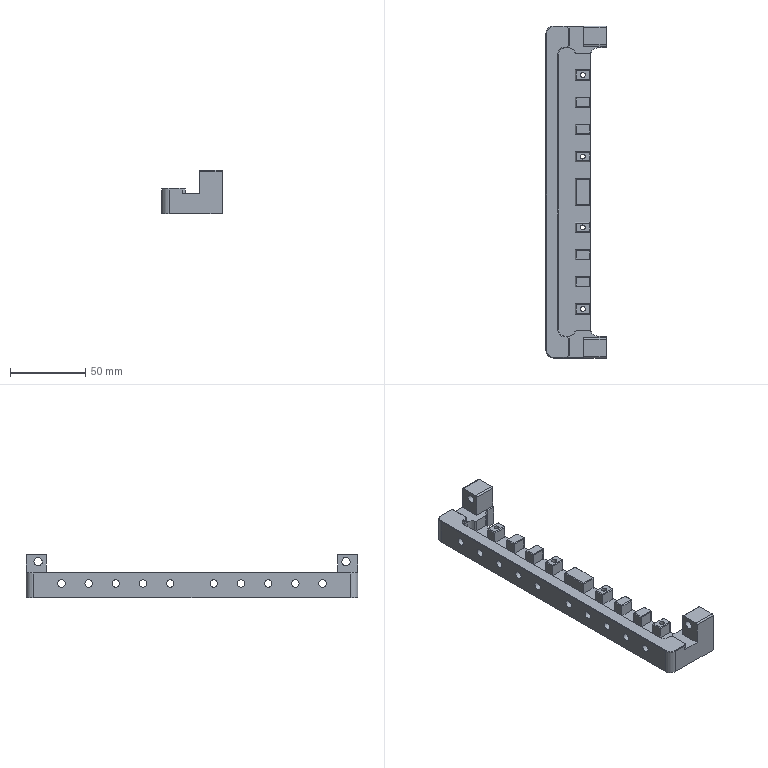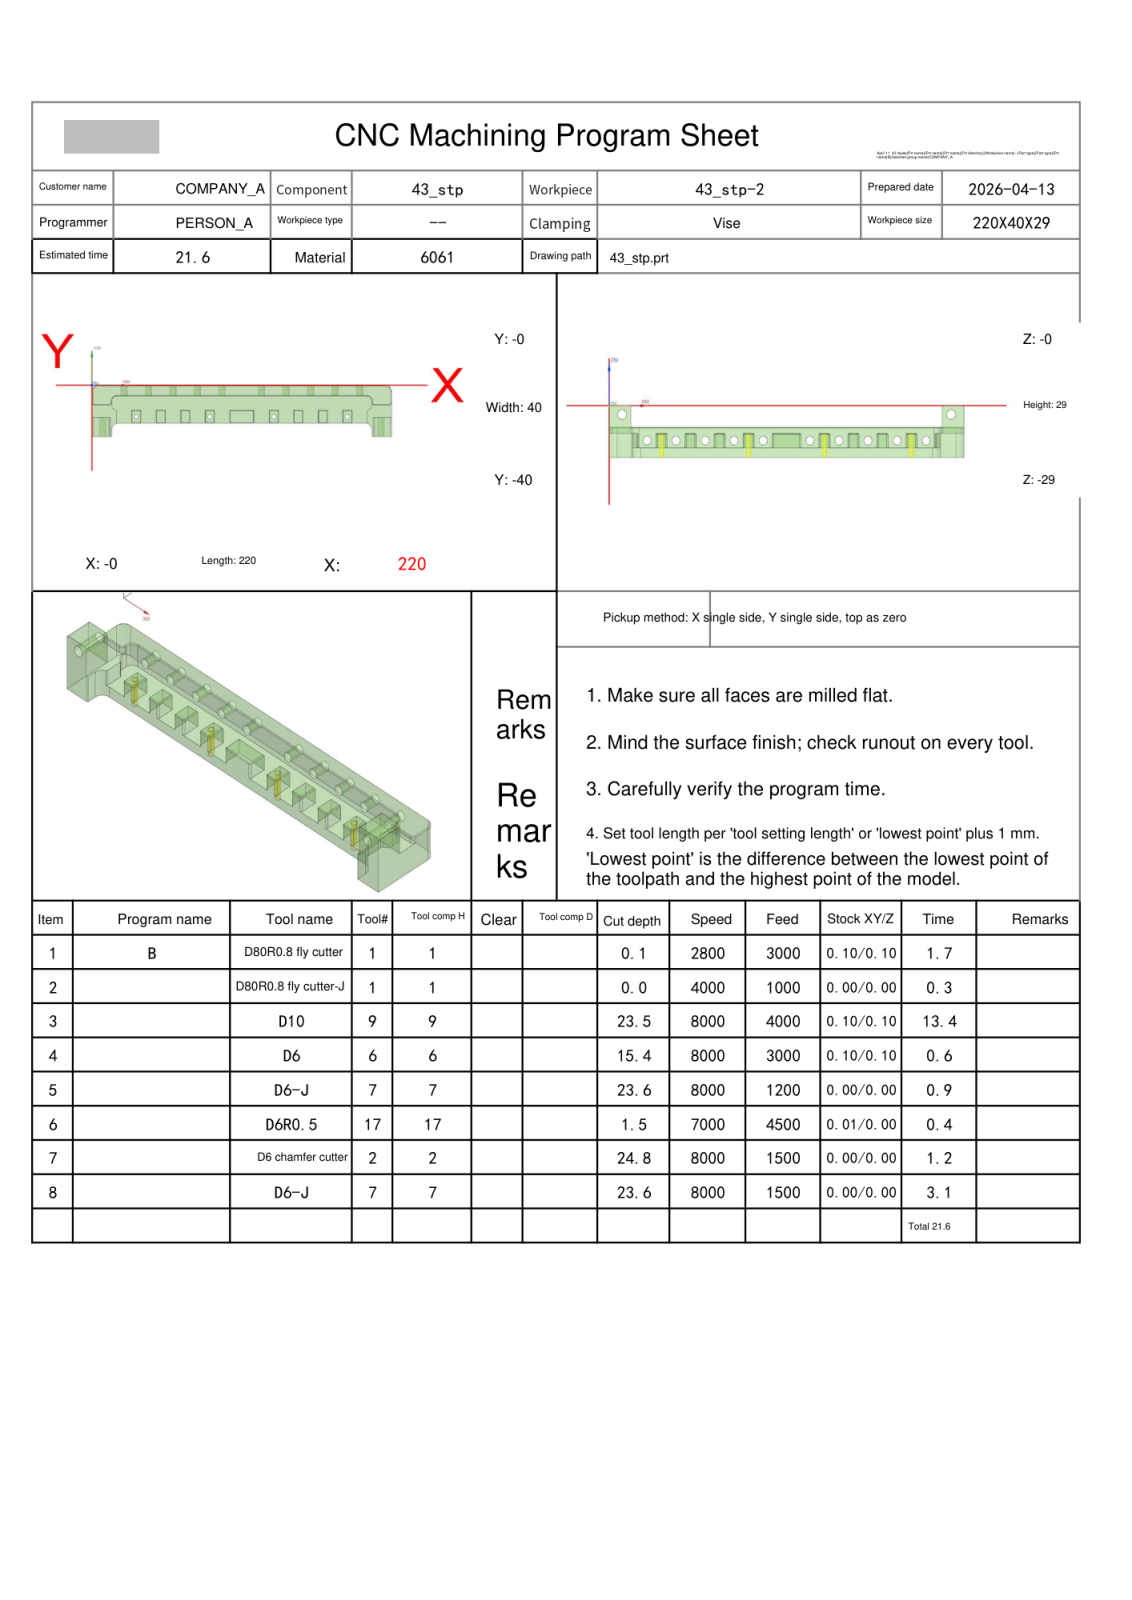NC program | NX | posted by the shop | part box 40 x 220 x 29 mm
Lines 135 to 1312 of 14837:
N3 T09 M06
(D10  D=10. R=0. H=09 ce=0.10 di=0.10)
G00 G90 G54 X110. Y7.5 M03 S8000
G43 H09 Z15.8
M08
Z.905
G01 Z-.595 F4000.
Y4.4
X215.
G02 X224.4 Y-5. I0.0 J-9.4
G01 Y-8.601
X224.9
Y-19.9
X220.403
X201.4
Y-44.9
X200.6
Y-40.296
X198.686 Y-39.233
X196.695 Y-38.128
G02 X196.243 Y-37.538 I.453 J.816
G01 X195.952 Y-36.374
G03 X195.735 Y-35.959 I-.97 J-.243
G02 X195.462 Y-35.581 I1.882 J1.646
G01 X192.575 Y-30.673
G02 X192.23 Y-29.406 I2.155 J1.267
X194.73 Y-26.906 I2.5 J0.0
X196.885 Y-28.138 I0.0 J-2.5
G01 X199.772 Y-33.046
G02 X200.117 Y-34.313 I-2.155 J-1.267
X197.617 Y-36.813 I-2.5 J0.0
X197.203 Y-36.779 I0.0 J2.5
G01 X197.049 Y-36.766
G03 X196.762 Y-36.811 I0.0 J-.934
G01 X195.633 Y-37.175
G02 X195.326 Y-37.223 I-.307 J.952
X194.841 Y-37.098 I0.0 J1.
G01 X190.233 Y-34.539
X189.082 Y-33.9
X185.05
G02 X184.259 Y-33.842 I0.0 J5.4
X183.967 Y-33.79 I.791 J5.342
G01 X173.023 Y-33.792
G02 X171.95 Y-33.9 I-1.073 J5.292
G01 X167.05
G02 X166.259 Y-33.842 I0.0 J5.4
X165.967 Y-33.79 I.79 J5.342
G01 X155.023 Y-33.792
G02 X153.95 Y-33.9 I-1.073 J5.292
G01 X149.05
G02 X148.259 Y-33.842 I0.0 J5.4
X147.967 Y-33.79 I.79 J5.342
G01 X137.023 Y-33.792
G02 X135.95 Y-33.9 I-1.073 J5.292
G01 X131.05
G02 X130.259 Y-33.842 I0.0 J5.4
X129.967 Y-33.79 I.791 J5.342
G01 X119.023 Y-33.792
G02 X117.95 Y-33.9 I-1.073 J5.292
G01 X102.05
G02 X101.259 Y-33.842 I0.0 J5.4
X100.967 Y-33.79 I.79 J5.342
G01 X90.023 Y-33.792
G02 X88.95 Y-33.9 I-1.073 J5.292
G01 X84.05
G02 X83.259 Y-33.842 I0.0 J5.4
X82.967 Y-33.79 I.791 J5.342
G01 X72.023 Y-33.792
G02 X70.95 Y-33.9 I-1.073 J5.292
G01 X66.05
G02 X65.259 Y-33.842 I0.0 J5.4
X64.967 Y-33.79 I.791 J5.342
G01 X54.023 Y-33.792
G02 X52.95 Y-33.9 I-1.073 J5.292
G01 X48.05
G02 X47.26 Y-33.842 I0.0 J5.4
X46.968 Y-33.79 I.79 J5.342
G01 X36.023 Y-33.792
G02 X34.95 Y-33.9 I-1.073 J5.292
G01 X30.918
X25.134 Y-37.112
G02 X24.681 Y-37.229 I-.453 J.816
X24.394 Y-37.184 I0.0 J.934
G01 X23.253 Y-36.816
G03 X22.946 Y-36.767 I-.307 J-.952
G01 X22.786 Y-36.78
G02 X22.383 Y-36.813 I-.402 J2.467
X19.883 Y-34.313 I0.0 J2.5
X20.228 Y-33.046 I2.5 J0.0
G01 X23.115 Y-28.138
G02 X25.27 Y-26.906 I2.155 J-1.267
X27.77 Y-29.406 I0.0 J-2.5
X27.425 Y-30.673 I-2.5 J0.0
G01 X24.538 Y-35.58
G02 X24.257 Y-35.968 I-2.155 J1.267
G03 X24.052 Y-36.359 I.7 J-.618
G01 X23.764 Y-37.51
G02 X23.28 Y-38.141 I-.97 J.243
G01 X21.024 Y-39.394
X19.4 Y-40.296
Y-41.53
X18.6 Y-42.33
Y-19.9
X-4.9
Y-8.602
X-4.4
Y-5.
G02 X5. Y4.4 I9.4 J0.0
G01 X106.966
G02 X107.796 Y3.955 I-.001 J-1.
G01 X112.204 Y-2.655
G03 X113.035 Y-3.1 I.832 J.555
G01 X197.609
G02 X198.311 Y-3.388 I0.0 J-1.
G01 X199.813 Y-4.869
G03 X200.256 Y-5.122 I.702 J.712
G02 X202.109 Y-7.537 I-.647 J-2.415
X200.195 Y-9.967 I-2.5 J0.0
G01 X191.425 Y-12.084
G02 X190.838 Y-12.154 I-.587 J2.43
X188.338 Y-9.654 I0.0 J2.5
X190.252 Y-7.224 I2.5 J0.0
G01 X197.74 Y-5.416
G03 X198.255 Y-5.106 I-.235 J.972
G01 X199.727 Y-3.438
G02 X200.477 Y-3.1 I.75 J-.662
G01 X215.
G02 X216.9 Y-5. I0.0 J-1.9
G01 Y-8.601
G03 X217.32 Y-11.075 I7.5 J0.0
G02 X217.374 Y-11.4 I-.946 J-.325
X216.379 Y-12.4 I-1. J0.0
G01 X201.4
G03 X193.9 Y-19.9 I0.0 J-7.5
G01 Y-26.31
G02 X192.9 Y-27.306 I-1. J.004
X192.455 Y-27.201 I0.0 J1.
G03 X189.082 Y-26.4 I-3.372 J-6.699
G01 X185.357
X185.167 Y-26.381
X184.72 Y-26.29
X172.28
X171.833 Y-26.381
X171.643 Y-26.4
X167.357
X167.167 Y-26.381
X166.72 Y-26.29
X154.28
X153.833 Y-26.381
X153.643 Y-26.4
X149.357
X149.167 Y-26.381
X148.72 Y-26.29
X136.28
X135.833 Y-26.381
X135.643 Y-26.4
X131.357
X131.167 Y-26.381
X130.72 Y-26.29
X118.28
X117.833 Y-26.381
X117.643 Y-26.4
X102.357
X102.167 Y-26.381
X101.72 Y-26.29
X89.28
X88.833 Y-26.381
X88.643 Y-26.4
X84.357
X84.167 Y-26.381
X83.72 Y-26.29
X71.28
X70.833 Y-26.381
X70.643 Y-26.4
X66.357
X66.167 Y-26.381
X65.72 Y-26.29
X53.28
X52.833 Y-26.381
X52.643 Y-26.4
X48.356
X48.167 Y-26.381
X47.72 Y-26.29
X35.28
X34.833 Y-26.381
G02 X34.635 Y-26.401 I-.199 J.981
G01 X34.593 Y-26.4
X30.918
G03 X27.545 Y-27.201 I0.0 J-7.5
G02 X27.1 Y-27.306 I-.445 J.895
X26.1 Y-26.31 I0.0 J1.
G01 Y-19.9
G03 X18.6 Y-12.4 I-7.5 J0.0
G01 X3.622
G02 X2.626 Y-11.4 I.004 J1.
X2.681 Y-11.075 I1. J0.0
G03 X3.1 Y-8.602 I-7.081 J2.473
G01 Y-5.
G02 X5. Y-3.1 I1.9 J0.0
G01 X19.523
G02 X20.273 Y-3.438 I0.0 J-1.
G01 X21.745 Y-5.106
G03 X22.26 Y-5.416 I.75 J.662
G01 X29.748 Y-7.224
G02 X31.662 Y-9.654 I-.587 J-2.43
X29.162 Y-12.154 I-2.5 J0.0
X28.575 Y-12.084 I0.0 J2.5
G01 X19.805 Y-9.967
G02 X17.891 Y-7.537 I.587 J2.43
X19.744 Y-5.122 I2.5 J0.0
G03 X20.187 Y-4.868 I-.259 J.966
G01 X21.689 Y-3.388
G02 X22.391 Y-3.1 I.702 J-.712
G01 X106.965
G02 X107.796 Y-3.545 I-.001 J-1.
G01 X112.204 Y-10.155
G03 X113.035 Y-10.6 I.832 J.555
G01 X187.726
G02 X188.721 Y-11.6 I-.005 J-1.
X188.579 Y-12.115 I-1. J0.0
G03 X186.53 Y-17.929 I12.821 J-7.785
G02 X185.539 Y-18.793 I-.991 J.136
G01 X185.472 Y-18.79
X171.528
X171.08 Y-18.881
X170.891 Y-18.9
X168.109
X167.92 Y-18.881
X167.472 Y-18.79
X153.528
X153.08 Y-18.881
X152.891 Y-18.9
X150.109
X149.92 Y-18.881
X149.472 Y-18.79
X135.528
X135.08 Y-18.881
X134.891 Y-18.9
X132.109
X131.92 Y-18.881
X131.472 Y-18.79
X117.528
X117.08 Y-18.881
X116.891 Y-18.9
X103.109
X102.92 Y-18.881
X102.472 Y-18.79
X88.528
X88.08 Y-18.881
X87.891 Y-18.9
X85.109
X84.92 Y-18.881
X84.472 Y-18.79
X70.528
X70.08 Y-18.881
X69.891 Y-18.9
X67.109
X66.92 Y-18.881
X66.472 Y-18.79
X52.528
X52.08 Y-18.881
X51.891 Y-18.9
X49.108
X48.92 Y-18.881
X48.472 Y-18.79
X34.528
X34.461 Y-18.793
G02 X33.47 Y-17.929 I0.0 J1.
G03 X31.421 Y-12.115 I-14.87 J-1.971
G02 X31.279 Y-11.6 I.857 J.515
X32.274 Y-10.6 I1. J0.0
G01 X110.
X110.5
Y-7.6
Z.905
G00 X110. Y7.5
Z.31
G01 Z-1.19
Y4.4
X215.
G02 X224.4 Y-5. I0.0 J-9.4
G01 Y-8.601
X224.9
Y-19.9
X220.403
X201.4
Y-44.9
X200.6
Y-40.296
X198.686 Y-39.233
X196.695 Y-38.128
G02 X196.243 Y-37.538 I.453 J.816
G01 X195.952 Y-36.374
G03 X195.735 Y-35.959 I-.97 J-.243
G02 X195.462 Y-35.581 I1.882 J1.646
G01 X192.575 Y-30.673
G02 X192.23 Y-29.406 I2.155 J1.267
X194.73 Y-26.906 I2.5 J0.0
X196.885 Y-28.138 I0.0 J-2.5
G01 X199.772 Y-33.046
G02 X200.117 Y-34.313 I-2.155 J-1.267
X197.617 Y-36.813 I-2.5 J0.0
X197.203 Y-36.779 I0.0 J2.5
G01 X197.049 Y-36.766
G03 X196.762 Y-36.811 I0.0 J-.934
G01 X195.633 Y-37.175
G02 X195.326 Y-37.223 I-.307 J.952
X194.841 Y-37.098 I0.0 J1.
G01 X190.233 Y-34.539
X189.082 Y-33.9
X185.05
G02 X184.259 Y-33.842 I0.0 J5.4
X183.967 Y-33.79 I.791 J5.342
G01 X173.023 Y-33.792
G02 X171.95 Y-33.9 I-1.073 J5.292
G01 X167.05
G02 X166.259 Y-33.842 I0.0 J5.4
X165.967 Y-33.79 I.79 J5.342
G01 X155.023 Y-33.792
G02 X153.95 Y-33.9 I-1.073 J5.292
G01 X149.05
G02 X148.259 Y-33.842 I0.0 J5.4
X147.967 Y-33.79 I.79 J5.342
G01 X137.023 Y-33.792
G02 X135.95 Y-33.9 I-1.073 J5.292
G01 X131.05
G02 X130.259 Y-33.842 I0.0 J5.4
X129.967 Y-33.79 I.791 J5.342
G01 X119.023 Y-33.792
G02 X117.95 Y-33.9 I-1.073 J5.292
G01 X102.05
G02 X101.259 Y-33.842 I0.0 J5.4
X100.967 Y-33.79 I.79 J5.342
G01 X90.023 Y-33.792
G02 X88.95 Y-33.9 I-1.073 J5.292
G01 X84.05
G02 X83.259 Y-33.842 I0.0 J5.4
X82.967 Y-33.79 I.791 J5.342
G01 X72.023 Y-33.792
G02 X70.95 Y-33.9 I-1.073 J5.292
G01 X66.05
G02 X65.259 Y-33.842 I0.0 J5.4
X64.967 Y-33.79 I.791 J5.342
G01 X54.023 Y-33.792
G02 X52.95 Y-33.9 I-1.073 J5.292
G01 X48.05
G02 X47.26 Y-33.842 I0.0 J5.4
X46.968 Y-33.79 I.79 J5.342
G01 X36.023 Y-33.792
G02 X34.95 Y-33.9 I-1.073 J5.292
G01 X30.918
X25.134 Y-37.112
G02 X24.681 Y-37.229 I-.453 J.816
X24.394 Y-37.184 I0.0 J.934
G01 X23.253 Y-36.816
G03 X22.946 Y-36.767 I-.307 J-.952
G01 X22.786 Y-36.78
G02 X22.383 Y-36.813 I-.402 J2.467
X19.883 Y-34.313 I0.0 J2.5
X20.228 Y-33.046 I2.5 J0.0
G01 X23.115 Y-28.138
G02 X25.27 Y-26.906 I2.155 J-1.267
X27.77 Y-29.406 I0.0 J-2.5
X27.425 Y-30.673 I-2.5 J0.0
G01 X24.538 Y-35.58
G02 X24.257 Y-35.968 I-2.155 J1.267
G03 X24.052 Y-36.359 I.7 J-.618
G01 X23.764 Y-37.51
G02 X23.28 Y-38.141 I-.97 J.243
G01 X21.024 Y-39.394
X19.4 Y-40.296
Y-41.53
X18.6 Y-42.33
Y-19.9
X-4.9
Y-8.602
X-4.4
Y-5.
G02 X5. Y4.4 I9.4 J0.0
G01 X106.966
G02 X107.796 Y3.955 I-.001 J-1.
G01 X112.204 Y-2.655
G03 X113.035 Y-3.1 I.832 J.555
G01 X197.609
G02 X198.311 Y-3.388 I0.0 J-1.
G01 X199.813 Y-4.869
G03 X200.256 Y-5.122 I.702 J.712
G02 X202.109 Y-7.537 I-.647 J-2.415
X200.195 Y-9.967 I-2.5 J0.0
G01 X191.425 Y-12.084
G02 X190.838 Y-12.154 I-.587 J2.43
X188.338 Y-9.654 I0.0 J2.5
X190.252 Y-7.224 I2.5 J0.0
G01 X197.74 Y-5.416
G03 X198.255 Y-5.106 I-.235 J.972
G01 X199.727 Y-3.438
G02 X200.477 Y-3.1 I.75 J-.662
G01 X215.
G02 X216.9 Y-5. I0.0 J-1.9
G01 Y-8.601
G03 X217.32 Y-11.075 I7.5 J0.0
G02 X217.374 Y-11.4 I-.946 J-.325
X216.379 Y-12.4 I-1. J0.0
G01 X201.4
G03 X193.9 Y-19.9 I0.0 J-7.5
G01 Y-26.31
G02 X192.9 Y-27.306 I-1. J.004
X192.455 Y-27.201 I0.0 J1.
G03 X189.082 Y-26.4 I-3.372 J-6.699
G01 X185.357
X185.167 Y-26.381
X184.72 Y-26.29
X172.28
X171.833 Y-26.381
X171.643 Y-26.4
X167.357
X167.167 Y-26.381
X166.72 Y-26.29
X154.28
X153.833 Y-26.381
X153.643 Y-26.4
X149.357
X149.167 Y-26.381
X148.72 Y-26.29
X136.28
X135.833 Y-26.381
X135.643 Y-26.4
X131.357
X131.167 Y-26.381
X130.72 Y-26.29
X118.28
X117.833 Y-26.381
X117.643 Y-26.4
X102.357
X102.167 Y-26.381
X101.72 Y-26.29
X89.28
X88.833 Y-26.381
X88.643 Y-26.4
X84.357
X84.167 Y-26.381
X83.72 Y-26.29
X71.28
X70.833 Y-26.381
X70.643 Y-26.4
X66.357
X66.167 Y-26.381
X65.72 Y-26.29
X53.28
X52.833 Y-26.381
X52.643 Y-26.4
X48.356
X48.167 Y-26.381
X47.72 Y-26.29
X35.28
X34.833 Y-26.381
G02 X34.635 Y-26.401 I-.199 J.981
G01 X34.593 Y-26.4
X30.918
G03 X27.545 Y-27.201 I0.0 J-7.5
G02 X27.1 Y-27.306 I-.445 J.895
X26.1 Y-26.31 I0.0 J1.
G01 Y-19.9
G03 X18.6 Y-12.4 I-7.5 J0.0
G01 X3.622
G02 X2.626 Y-11.4 I.004 J1.
X2.681 Y-11.075 I1. J0.0
G03 X3.1 Y-8.602 I-7.081 J2.473
G01 Y-5.
G02 X5. Y-3.1 I1.9 J0.0
G01 X19.523
G02 X20.273 Y-3.438 I0.0 J-1.
G01 X21.745 Y-5.106
G03 X22.26 Y-5.416 I.75 J.662
G01 X29.748 Y-7.224
G02 X31.662 Y-9.654 I-.587 J-2.43
X29.162 Y-12.154 I-2.5 J0.0
X28.575 Y-12.084 I0.0 J2.5
G01 X19.805 Y-9.967
G02 X17.891 Y-7.537 I.587 J2.43
X19.744 Y-5.122 I2.5 J0.0
G03 X20.187 Y-4.868 I-.259 J.966
G01 X21.689 Y-3.388
G02 X22.391 Y-3.1 I.702 J-.712
G01 X106.965
G02 X107.796 Y-3.545 I-.001 J-1.
G01 X112.204 Y-10.155
G03 X113.035 Y-10.6 I.832 J.555
G01 X187.726
G02 X188.721 Y-11.6 I-.005 J-1.
X188.579 Y-12.115 I-1. J0.0
G03 X186.53 Y-17.929 I12.821 J-7.785
G02 X185.539 Y-18.793 I-.991 J.136
G01 X185.472 Y-18.79
X171.528
X171.08 Y-18.881
X170.891 Y-18.9
X168.109
X167.92 Y-18.881
X167.472 Y-18.79
X153.528
X153.08 Y-18.881
X152.891 Y-18.9
X150.109
X149.92 Y-18.881
X149.472 Y-18.79
X135.528
X135.08 Y-18.881
X134.891 Y-18.9
X132.109
X131.92 Y-18.881
X131.472 Y-18.79
X117.528
X117.08 Y-18.881
X116.891 Y-18.9
X103.109
X102.92 Y-18.881
X102.472 Y-18.79
X88.528
X88.08 Y-18.881
X87.891 Y-18.9
X85.109
X84.92 Y-18.881
X84.472 Y-18.79
X70.528
X70.08 Y-18.881
X69.891 Y-18.9
X67.109
X66.92 Y-18.881
X66.472 Y-18.79
X52.528
X52.08 Y-18.881
X51.891 Y-18.9
X49.108
X48.92 Y-18.881
X48.472 Y-18.79
X34.528
X34.461 Y-18.793
G02 X33.47 Y-17.929 I0.0 J1.
G03 X31.421 Y-12.115 I-14.87 J-1.971
G02 X31.279 Y-11.6 I.857 J.515
X32.274 Y-10.6 I1. J0.0
G01 X110.
X110.5
Y-7.6
Z.31
G00 X110. Y7.5
Z-.285
G01 Z-1.785
Y4.4
X215.
G02 X224.4 Y-5. I0.0 J-9.4
G01 Y-8.601
X224.9
Y-19.9
X220.403
X201.4
Y-44.9
X200.6
Y-40.296
X198.686 Y-39.233
X196.695 Y-38.128
G02 X196.243 Y-37.538 I.453 J.816
G01 X195.952 Y-36.374
G03 X195.735 Y-35.959 I-.97 J-.243
G02 X195.462 Y-35.581 I1.882 J1.646
G01 X192.575 Y-30.673
G02 X192.23 Y-29.406 I2.155 J1.267
X194.73 Y-26.906 I2.5 J0.0
X196.885 Y-28.138 I0.0 J-2.5
G01 X199.772 Y-33.046
G02 X200.117 Y-34.313 I-2.155 J-1.267
X197.617 Y-36.813 I-2.5 J0.0
X197.203 Y-36.779 I0.0 J2.5
G01 X197.049 Y-36.766
G03 X196.762 Y-36.811 I0.0 J-.934
G01 X195.633 Y-37.175
G02 X195.326 Y-37.223 I-.307 J.952
X194.841 Y-37.098 I0.0 J1.
G01 X190.233 Y-34.539
X189.082 Y-33.9
X185.05
G02 X184.259 Y-33.842 I0.0 J5.4
X183.967 Y-33.79 I.791 J5.342
G01 X173.023 Y-33.792
G02 X171.95 Y-33.9 I-1.073 J5.292
G01 X167.05
G02 X166.259 Y-33.842 I0.0 J5.4
X165.967 Y-33.79 I.79 J5.342
G01 X155.023 Y-33.792
G02 X153.95 Y-33.9 I-1.073 J5.292
G01 X149.05
G02 X148.259 Y-33.842 I0.0 J5.4
X147.967 Y-33.79 I.79 J5.342
G01 X137.023 Y-33.792
G02 X135.95 Y-33.9 I-1.073 J5.292
G01 X131.05
G02 X130.259 Y-33.842 I0.0 J5.4
X129.967 Y-33.79 I.791 J5.342
G01 X119.023 Y-33.792
G02 X117.95 Y-33.9 I-1.073 J5.292
G01 X102.05
G02 X101.259 Y-33.842 I0.0 J5.4
X100.967 Y-33.79 I.79 J5.342
G01 X90.023 Y-33.792
G02 X88.95 Y-33.9 I-1.073 J5.292
G01 X84.05
G02 X83.259 Y-33.842 I0.0 J5.4
X82.967 Y-33.79 I.791 J5.342
G01 X72.023 Y-33.792
G02 X70.95 Y-33.9 I-1.073 J5.292
G01 X66.05
G02 X65.259 Y-33.842 I0.0 J5.4
X64.967 Y-33.79 I.791 J5.342
G01 X54.023 Y-33.792
G02 X52.95 Y-33.9 I-1.073 J5.292
G01 X48.05
G02 X47.26 Y-33.842 I0.0 J5.4
X46.968 Y-33.79 I.79 J5.342
G01 X36.023 Y-33.792
G02 X34.95 Y-33.9 I-1.073 J5.292
G01 X30.918
X25.134 Y-37.112
G02 X24.681 Y-37.229 I-.453 J.816
X24.394 Y-37.184 I0.0 J.934
G01 X23.253 Y-36.816
G03 X22.946 Y-36.767 I-.307 J-.952
G01 X22.786 Y-36.78
G02 X22.383 Y-36.813 I-.402 J2.467
X19.883 Y-34.313 I0.0 J2.5
X20.228 Y-33.046 I2.5 J0.0
G01 X23.115 Y-28.138
G02 X25.27 Y-26.906 I2.155 J-1.267
X27.77 Y-29.406 I0.0 J-2.5
X27.425 Y-30.673 I-2.5 J0.0
G01 X24.538 Y-35.58
G02 X24.257 Y-35.968 I-2.155 J1.267
G03 X24.052 Y-36.359 I.7 J-.618
G01 X23.764 Y-37.51
G02 X23.28 Y-38.141 I-.97 J.243
G01 X21.024 Y-39.394
X19.4 Y-40.296
Y-41.53
X18.6 Y-42.33
Y-19.9
X-4.9
Y-8.602
X-4.4
Y-5.
G02 X5. Y4.4 I9.4 J0.0
G01 X106.966
G02 X107.796 Y3.955 I-.001 J-1.
G01 X112.204 Y-2.655
G03 X113.035 Y-3.1 I.832 J.555
G01 X197.609
G02 X198.311 Y-3.388 I0.0 J-1.
G01 X199.813 Y-4.869
G03 X200.256 Y-5.122 I.702 J.712
G02 X202.109 Y-7.537 I-.647 J-2.415
X200.195 Y-9.967 I-2.5 J0.0
G01 X191.425 Y-12.084
G02 X190.838 Y-12.154 I-.587 J2.43
X188.338 Y-9.654 I0.0 J2.5
X190.252 Y-7.224 I2.5 J0.0
G01 X197.74 Y-5.416
G03 X198.255 Y-5.106 I-.235 J.972
G01 X199.727 Y-3.438
G02 X200.477 Y-3.1 I.75 J-.662
G01 X215.
G02 X216.9 Y-5. I0.0 J-1.9
G01 Y-8.601
G03 X217.32 Y-11.075 I7.5 J0.0
G02 X217.374 Y-11.4 I-.946 J-.325
X216.379 Y-12.4 I-1. J0.0
G01 X201.4
G03 X193.9 Y-19.9 I0.0 J-7.5
G01 Y-26.31
G02 X192.9 Y-27.306 I-1. J.004
X192.455 Y-27.201 I0.0 J1.
G03 X189.082 Y-26.4 I-3.372 J-6.699
G01 X185.357
X185.167 Y-26.381
X184.72 Y-26.29
X172.28
X171.833 Y-26.381
X171.643 Y-26.4
X167.357
X167.167 Y-26.381
X166.72 Y-26.29
X154.28
X153.833 Y-26.381
X153.643 Y-26.4
X149.357
X149.167 Y-26.381
X148.72 Y-26.29
X136.28
X135.833 Y-26.381
X135.643 Y-26.4
X131.357
X131.167 Y-26.381
X130.72 Y-26.29
X118.28
X117.833 Y-26.381
X117.643 Y-26.4
X102.357
X102.167 Y-26.381
X101.72 Y-26.29
X89.28
X88.833 Y-26.381
X88.643 Y-26.4
X84.357
X84.167 Y-26.381
X83.72 Y-26.29
X71.28
X70.833 Y-26.381
X70.643 Y-26.4
X66.357
X66.167 Y-26.381
X65.72 Y-26.29
X53.28
X52.833 Y-26.381
X52.643 Y-26.4
X48.356
X48.167 Y-26.381
X47.72 Y-26.29
X35.28
X34.833 Y-26.381
G02 X34.635 Y-26.401 I-.199 J.981
G01 X34.593 Y-26.4
X30.918
G03 X27.545 Y-27.201 I0.0 J-7.5
G02 X27.1 Y-27.306 I-.445 J.895
X26.1 Y-26.31 I0.0 J1.
G01 Y-19.9
G03 X18.6 Y-12.4 I-7.5 J0.0
G01 X3.622
G02 X2.626 Y-11.4 I.004 J1.
X2.681 Y-11.075 I1. J0.0
G03 X3.1 Y-8.602 I-7.081 J2.473
G01 Y-5.
G02 X5. Y-3.1 I1.9 J0.0
G01 X19.523
G02 X20.273 Y-3.438 I0.0 J-1.
G01 X21.745 Y-5.106
G03 X22.26 Y-5.416 I.75 J.662
G01 X29.748 Y-7.224
G02 X31.662 Y-9.654 I-.587 J-2.43
X29.162 Y-12.154 I-2.5 J0.0
X28.575 Y-12.084 I0.0 J2.5
G01 X19.805 Y-9.967
G02 X17.891 Y-7.537 I.587 J2.43
X19.744 Y-5.122 I2.5 J0.0
G03 X20.187 Y-4.868 I-.259 J.966
G01 X21.689 Y-3.388
G02 X22.391 Y-3.1 I.702 J-.712
G01 X106.965
G02 X107.796 Y-3.545 I-.001 J-1.
G01 X112.204 Y-10.155
G03 X113.035 Y-10.6 I.832 J.555
G01 X187.726
G02 X188.721 Y-11.6 I-.005 J-1.
X188.579 Y-12.115 I-1. J0.0
G03 X186.53 Y-17.929 I12.821 J-7.785
G02 X185.539 Y-18.793 I-.991 J.136
G01 X185.472 Y-18.79
X171.528
X171.08 Y-18.881
X170.891 Y-18.9
X168.109
X167.92 Y-18.881
X167.472 Y-18.79
X153.528
X153.08 Y-18.881
X152.891 Y-18.9
X150.109
X149.92 Y-18.881
X149.472 Y-18.79
X135.528
X135.08 Y-18.881
X134.891 Y-18.9
X132.109
X131.92 Y-18.881
X131.472 Y-18.79
X117.528
X117.08 Y-18.881
X116.891 Y-18.9
X103.109
X102.92 Y-18.881
X102.472 Y-18.79
X88.528
X88.08 Y-18.881
X87.891 Y-18.9
X85.109
X84.92 Y-18.881
X84.472 Y-18.79
X70.528
X70.08 Y-18.881
X69.891 Y-18.9
X67.109
X66.92 Y-18.881
X66.472 Y-18.79
X52.528
X52.08 Y-18.881
X51.891 Y-18.9
X49.108
X48.92 Y-18.881
X48.472 Y-18.79
X34.528
X34.461 Y-18.793
G02 X33.47 Y-17.929 I0.0 J1.
G03 X31.421 Y-12.115 I-14.87 J-1.971
G02 X31.279 Y-11.6 I.857 J.515
X32.274 Y-10.6 I1. J0.0
G01 X110.
X110.5
Y-7.6
Z-.285
G00 X110. Y7.5
Z-.88
G01 Z-2.38
Y4.4
X215.
G02 X224.4 Y-5. I0.0 J-9.4
G01 Y-8.601
X224.9
Y-19.9
X220.403
X201.4
Y-44.9
X200.6
Y-40.296
X198.686 Y-39.233
X196.695 Y-38.128
G02 X196.243 Y-37.538 I.453 J.816
G01 X195.952 Y-36.374
G03 X195.735 Y-35.959 I-.97 J-.243
G02 X195.462 Y-35.581 I1.882 J1.646
G01 X192.575 Y-30.673
G02 X192.23 Y-29.406 I2.155 J1.267
X194.73 Y-26.906 I2.5 J0.0
X196.885 Y-28.138 I0.0 J-2.5
G01 X199.772 Y-33.046
G02 X200.117 Y-34.313 I-2.155 J-1.267
X197.617 Y-36.813 I-2.5 J0.0
X197.203 Y-36.779 I0.0 J2.5
G01 X197.049 Y-36.766
G03 X196.762 Y-36.811 I0.0 J-.934
G01 X195.633 Y-37.175
G02 X195.326 Y-37.223 I-.307 J.952
X194.841 Y-37.098 I0.0 J1.
G01 X190.233 Y-34.539
X189.082 Y-33.9
X185.05
G02 X184.259 Y-33.842 I0.0 J5.4
X183.967 Y-33.79 I.791 J5.342
G01 X173.023 Y-33.792
G02 X171.95 Y-33.9 I-1.073 J5.292
G01 X167.05
G02 X166.259 Y-33.842 I0.0 J5.4
X165.967 Y-33.79 I.79 J5.342
G01 X155.023 Y-33.792
G02 X153.95 Y-33.9 I-1.073 J5.292
G01 X149.05
G02 X148.259 Y-33.842 I0.0 J5.4
X147.967 Y-33.79 I.79 J5.342
G01 X137.023 Y-33.792
G02 X135.95 Y-33.9 I-1.073 J5.292
G01 X131.05
G02 X130.259 Y-33.842 I0.0 J5.4
X129.967 Y-33.79 I.791 J5.342
G01 X119.023 Y-33.792
G02 X117.95 Y-33.9 I-1.073 J5.292
G01 X102.05
G02 X101.259 Y-33.842 I0.0 J5.4
X100.967 Y-33.79 I.79 J5.342
G01 X90.023 Y-33.792
G02 X88.95 Y-33.9 I-1.073 J5.292
G01 X84.05
G02 X83.259 Y-33.842 I0.0 J5.4
X82.967 Y-33.79 I.791 J5.342
G01 X72.023 Y-33.792
G02 X70.95 Y-33.9 I-1.073 J5.292
G01 X66.05
G02 X65.259 Y-33.842 I0.0 J5.4
X64.967 Y-33.79 I.791 J5.342
G01 X54.023 Y-33.792
G02 X52.95 Y-33.9 I-1.073 J5.292
G01 X48.05
G02 X47.26 Y-33.842 I0.0 J5.4
X46.968 Y-33.79 I.79 J5.342
G01 X36.023 Y-33.792
G02 X34.95 Y-33.9 I-1.073 J5.292
G01 X30.918
X25.134 Y-37.112
G02 X24.681 Y-37.229 I-.453 J.816
X24.394 Y-37.184 I0.0 J.934
G01 X23.253 Y-36.816
G03 X22.946 Y-36.767 I-.307 J-.952
G01 X22.786 Y-36.78
G02 X22.383 Y-36.813 I-.402 J2.467
X19.883 Y-34.313 I0.0 J2.5
X20.228 Y-33.046 I2.5 J0.0
G01 X23.115 Y-28.138
G02 X25.27 Y-26.906 I2.155 J-1.267
X27.77 Y-29.406 I0.0 J-2.5
X27.425 Y-30.673 I-2.5 J0.0
G01 X24.538 Y-35.58
G02 X24.257 Y-35.968 I-2.155 J1.267
G03 X24.052 Y-36.359 I.7 J-.618
G01 X23.764 Y-37.51
G02 X23.28 Y-38.141 I-.97 J.243
G01 X21.024 Y-39.394
X19.4 Y-40.296
Y-41.53
X18.6 Y-42.33
Y-19.9
X-4.9
Y-8.602
X-4.4
Y-5.
G02 X5. Y4.4 I9.4 J0.0
G01 X106.966
G02 X107.796 Y3.955 I-.001 J-1.
G01 X112.204 Y-2.655
G03 X113.035 Y-3.1 I.832 J.555
G01 X197.609
G02 X198.311 Y-3.388 I0.0 J-1.
G01 X199.813 Y-4.869
G03 X200.256 Y-5.122 I.702 J.712
G02 X202.109 Y-7.537 I-.647 J-2.415
X200.195 Y-9.967 I-2.5 J0.0
G01 X191.425 Y-12.084
G02 X190.838 Y-12.154 I-.587 J2.43
X188.338 Y-9.654 I0.0 J2.5
X190.252 Y-7.224 I2.5 J0.0
G01 X197.74 Y-5.416
G03 X198.255 Y-5.106 I-.235 J.972
G01 X199.727 Y-3.438
G02 X200.477 Y-3.1 I.75 J-.662
G01 X215.
G02 X216.9 Y-5. I0.0 J-1.9
G01 Y-8.601
G03 X217.32 Y-11.075 I7.5 J0.0
G02 X217.374 Y-11.4 I-.946 J-.325
X216.379 Y-12.4 I-1. J0.0
G01 X201.4
G03 X193.9 Y-19.9 I0.0 J-7.5
G01 Y-26.31
G02 X192.9 Y-27.306 I-1. J.004
X192.455 Y-27.201 I0.0 J1.
G03 X189.082 Y-26.4 I-3.372 J-6.699
G01 X185.357
X185.167 Y-26.381
X184.72 Y-26.29
X172.28
X171.833 Y-26.381
X171.643 Y-26.4
X167.357
X167.167 Y-26.381
X166.72 Y-26.29
X154.28
X153.833 Y-26.381
X153.643 Y-26.4
X149.357
X149.167 Y-26.381
X148.72 Y-26.29
X136.28
X135.833 Y-26.381
X135.643 Y-26.4
X131.357
X131.167 Y-26.381
X130.72 Y-26.29
X118.28
X117.833 Y-26.381
X117.643 Y-26.4
X102.357
X102.167 Y-26.381
X101.72 Y-26.29
X89.28
X88.833 Y-26.381
X88.643 Y-26.4
X84.357
X84.167 Y-26.381
X83.72 Y-26.29
X71.28
X70.833 Y-26.381
X70.643 Y-26.4
X66.357
X66.167 Y-26.381
X65.72 Y-26.29
X53.28
X52.833 Y-26.381
X52.643 Y-26.4
X48.356
X48.167 Y-26.381
X47.72 Y-26.29
X35.28
X34.833 Y-26.381
G02 X34.635 Y-26.401 I-.199 J.981
G01 X34.593 Y-26.4
X30.918
G03 X27.545 Y-27.201 I0.0 J-7.5
G02 X27.1 Y-27.306 I-.445 J.895
X26.1 Y-26.31 I0.0 J1.
G01 Y-19.9
G03 X18.6 Y-12.4 I-7.5 J0.0
G01 X3.622
G02 X2.626 Y-11.4 I.004 J1.
X2.681 Y-11.075 I1. J0.0
G03 X3.1 Y-8.602 I-7.081 J2.473
G01 Y-5.
G02 X5. Y-3.1 I1.9 J0.0
G01 X19.523
G02 X20.273 Y-3.438 I0.0 J-1.
G01 X21.745 Y-5.106
G03 X22.26 Y-5.416 I.75 J.662
G01 X29.748 Y-7.224
G02 X31.662 Y-9.654 I-.587 J-2.43
X29.162 Y-12.154 I-2.5 J0.0
X28.575 Y-12.084 I0.0 J2.5
G01 X19.805 Y-9.967
G02 X17.891 Y-7.537 I.587 J2.43
X19.744 Y-5.122 I2.5 J0.0
G03 X20.187 Y-4.868 I-.259 J.966
G01 X21.689 Y-3.388
G02 X22.391 Y-3.1 I.702 J-.712
G01 X106.965
G02 X107.796 Y-3.545 I-.001 J-1.
G01 X112.204 Y-10.155
G03 X113.035 Y-10.6 I.832 J.555
G01 X187.726
G02 X188.721 Y-11.6 I-.005 J-1.
X188.579 Y-12.115 I-1. J0.0
G03 X186.53 Y-17.929 I12.821 J-7.785
G02 X185.539 Y-18.793 I-.991 J.136
G01 X185.472 Y-18.79
X171.528
X171.08 Y-18.881
X170.891 Y-18.9
X168.109
X167.92 Y-18.881
X167.472 Y-18.79
X153.528
X153.08 Y-18.881
X152.891 Y-18.9
X150.109
X149.92 Y-18.881
X149.472 Y-18.79
X135.528
X135.08 Y-18.881
X134.891 Y-18.9
X132.109
X131.92 Y-18.881
X131.472 Y-18.79
X117.528
X117.08 Y-18.881
X116.891 Y-18.9
X103.109
X102.92 Y-18.881
X102.472 Y-18.79
X88.528
X88.08 Y-18.881
X87.891 Y-18.9
X85.109
X84.92 Y-18.881
X84.472 Y-18.79
X70.528
X70.08 Y-18.881
X69.891 Y-18.9
X67.109
X66.92 Y-18.881
X66.472 Y-18.79
X52.528
X52.08 Y-18.881
X51.891 Y-18.9
X49.108
X48.92 Y-18.881
X48.472 Y-18.79
X34.528
X34.461 Y-18.793
G02 X33.47 Y-17.929 I0.0 J1.
G03 X31.421 Y-12.115 I-14.87 J-1.971
G02 X31.279 Y-11.6 I.857 J.515
X32.274 Y-10.6 I1. J0.0
G01 X110.
X110.5
Y-7.6
Z-.88
G00 X110. Y7.5
Z-1.475
G01 Z-2.975
Y4.4
X215.
G02 X224.4 Y-5. I0.0 J-9.4
G01 Y-8.601
X224.9
Y-19.9
X220.403
X201.4
Y-44.9
X200.6
Y-40.296
X198.686 Y-39.233
X196.695 Y-38.128
G02 X196.243 Y-37.538 I.453 J.816
G01 X195.952 Y-36.374
G03 X195.735 Y-35.959 I-.97 J-.243
G02 X195.462 Y-35.581 I1.882 J1.646
G01 X192.575 Y-30.673
G02 X192.23 Y-29.406 I2.155 J1.267
X194.73 Y-26.906 I2.5 J0.0
X196.885 Y-28.138 I0.0 J-2.5
G01 X199.772 Y-33.046
G02 X200.117 Y-34.313 I-2.155 J-1.267
X197.617 Y-36.813 I-2.5 J0.0
X197.203 Y-36.779 I0.0 J2.5
G01 X197.049 Y-36.766
G03 X196.762 Y-36.811 I0.0 J-.934
G01 X195.633 Y-37.175
G02 X195.326 Y-37.223 I-.307 J.952
X194.841 Y-37.098 I0.0 J1.
G01 X190.233 Y-34.539
X189.082 Y-33.9
X185.05
G02 X184.259 Y-33.842 I0.0 J5.4
X183.967 Y-33.79 I.791 J5.342
G01 X173.023 Y-33.792
G02 X171.95 Y-33.9 I-1.073 J5.292
G01 X167.05
G02 X166.259 Y-33.842 I0.0 J5.4
X165.967 Y-33.79 I.79 J5.342
G01 X155.023 Y-33.792
G02 X153.95 Y-33.9 I-1.073 J5.292
G01 X149.05
G02 X148.259 Y-33.842 I0.0 J5.4
X147.967 Y-33.79 I.79 J5.342
G01 X137.023 Y-33.792
G02 X135.95 Y-33.9 I-1.073 J5.292
G01 X131.05
G02 X130.259 Y-33.842 I0.0 J5.4
X129.967 Y-33.79 I.791 J5.342
G01 X119.023 Y-33.792
G02 X117.95 Y-33.9 I-1.073 J5.292
G01 X102.05
G02 X101.259 Y-33.842 I0.0 J5.4
X100.967 Y-33.79 I.79 J5.342
G01 X90.023 Y-33.792
G02 X88.95 Y-33.9 I-1.073 J5.292
G01 X84.05
G02 X83.259 Y-33.842 I0.0 J5.4
X82.967 Y-33.79 I.791 J5.342
G01 X72.023 Y-33.792
G02 X70.95 Y-33.9 I-1.073 J5.292
G01 X66.05
G02 X65.259 Y-33.842 I0.0 J5.4
X64.967 Y-33.79 I.791 J5.342
G01 X54.023 Y-33.792
G02 X52.95 Y-33.9 I-1.073 J5.292
G01 X48.05
G02 X47.26 Y-33.842 I0.0 J5.4
X46.968 Y-33.79 I.79 J5.342
G01 X36.023 Y-33.792
G02 X34.95 Y-33.9 I-1.073 J5.292
G01 X30.918
X25.134 Y-37.112
G02 X24.681 Y-37.229 I-.453 J.816
X24.394 Y-37.184 I0.0 J.934
G01 X23.253 Y-36.816
G03 X22.946 Y-36.767 I-.307 J-.952
G01 X22.786 Y-36.78
G02 X22.383 Y-36.813 I-.402 J2.467
X19.883 Y-34.313 I0.0 J2.5
X20.228 Y-33.046 I2.5 J0.0
G01 X23.115 Y-28.138
G02 X25.27 Y-26.906 I2.155 J-1.267
X27.77 Y-29.406 I0.0 J-2.5
X27.425 Y-30.673 I-2.5 J0.0
G01 X24.538 Y-35.58